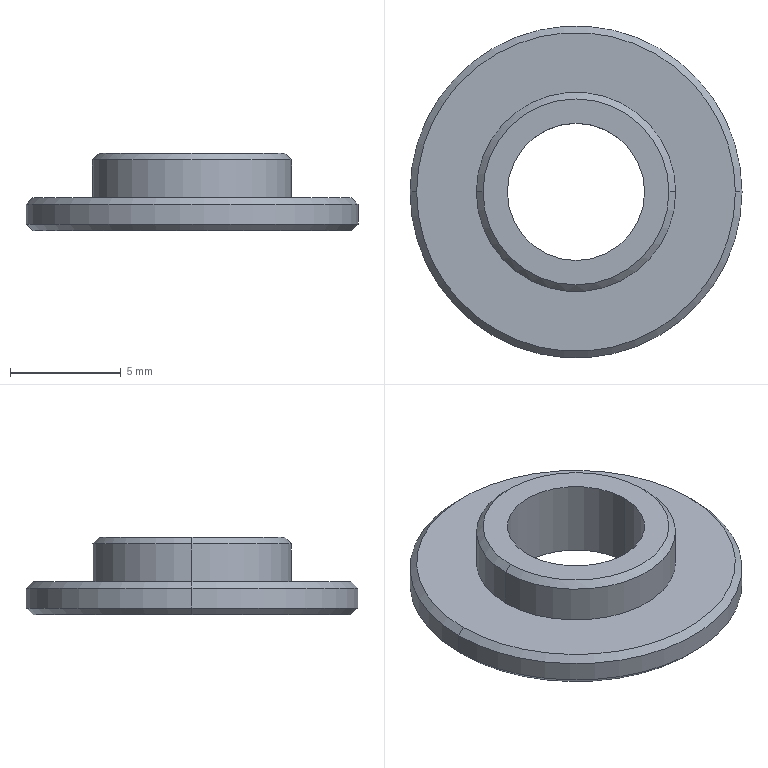Part | STEP file | 25 small sprocket spacer | 1 solid | 15 faces | box 15 x 15 x 3.5 mm | volume 281.21 mm3 | cone 6 | cylinder 6 | plane 3 | commonest cylinder face diameters 6.2 x2 9 x2 15 x2
STEP:
#1=CARTESIAN_POINT('',(0.,0.,0.));
#2=DIRECTION('',(0.,0.,1.));
#3=DIRECTION('',(1.,0.,0.));
#4=AXIS2_PLACEMENT_3D('',#1,#2,#3);
#5=CARTESIAN_POINT('',(-7.2,0.,0.));
#6=VERTEX_POINT('',#5);
#7=CARTESIAN_POINT('',(7.2,0.,0.));
#8=VERTEX_POINT('',#7);
#9=CARTESIAN_POINT('',(0.,0.,0.));
#10=DIRECTION('',(0.,0.,-1.));
#11=DIRECTION('',(1.,0.,0.));
#12=AXIS2_PLACEMENT_3D('',#9,#10,#11);
#13=CIRCLE('',#12,7.2);
#14=CARTESIAN_POINT('',(0.,0.,0.));
#15=DIRECTION('',(0.,0.,1.));
#16=DIRECTION('',(1.,0.,0.));
#17=AXIS2_PLACEMENT_3D('',#14,#15,#16);
#18=CONICAL_SURFACE('',#17,7.2,0.7854);
#19=CARTESIAN_POINT('',(6.283,0.));
#20=DIRECTION('',(-1.,0.));
#21=VECTOR('',#20,1.);
#22=LINE('',#19,#21);
#23=(GEOMETRIC_REPRESENTATION_CONTEXT(2)PARAMETRIC_REPRESENTATION_CONTEXT()REPRESENTATION_CONTEXT('',''));
#24=DEFINITIONAL_REPRESENTATION('',(#22),#23);
#25=PCURVE('',#18,#24);
#26=CARTESIAN_POINT('',(0.,0.,0.));
#27=DIRECTION('',(0.,0.,1.));
#28=DIRECTION('',(1.,0.,0.));
#29=AXIS2_PLACEMENT_3D('',#26,#27,#28);
#30=PLANE('',#29);
#31=CARTESIAN_POINT('',(7.2,0.));
#32=CARTESIAN_POINT('',(7.2,-12.471));
#33=CARTESIAN_POINT('',(-3.6,-6.235));
#34=CARTESIAN_POINT('',(-14.4,0.));
#35=CARTESIAN_POINT('',(-3.6,6.235));
#36=CARTESIAN_POINT('',(7.2,12.471));
#37=CARTESIAN_POINT('',(7.2,0.));
#38=(BOUNDED_CURVE()B_SPLINE_CURVE(2,(#31,#32,#33,#34,#35,#36,#37),.UNSPECIFIED.,.T.,.F.)B_SPLINE_CURVE_WITH_KNOTS((1,2,2,2,2,1),(-2.094,0.,2.094,4.189,6.283,8.378),.UNSPECIFIED.)CURVE()GEOMETRIC_REPRESENTATION_ITEM()RATIONAL_B_SPLINE_CURVE((1.,0.5,1.,0.5,1.,0.5,1.))REPRESENTATION_ITEM(''));
#39=(GEOMETRIC_REPRESENTATION_CONTEXT(2)PARAMETRIC_REPRESENTATION_CONTEXT()REPRESENTATION_CONTEXT('',''));
#40=DEFINITIONAL_REPRESENTATION('',(#38),#39);
#41=PCURVE('',#30,#40);
#42=SURFACE_CURVE('',#13,(#25,#41),.PCURVE_S1.);
#43=EDGE_CURVE('',#6,#8,#42,.T.);
#44=ORIENTED_EDGE('',*,*,#43,.F.);
#45=CARTESIAN_POINT('',(-7.5,0.,0.3));
#46=VERTEX_POINT('',#45);
#47=CARTESIAN_POINT('',(-7.2,0.,0.));
#48=DIRECTION('',(-0.7071,0.,0.7071));
#49=VECTOR('',#48,1.);
#50=LINE('',#47,#49);
#51=CARTESIAN_POINT('',(3.142,0.));
#52=DIRECTION('',(0.,1.));
#53=VECTOR('',#52,1.);
#54=LINE('',#51,#53);
#55=(GEOMETRIC_REPRESENTATION_CONTEXT(2)PARAMETRIC_REPRESENTATION_CONTEXT()REPRESENTATION_CONTEXT('',''));
#56=DEFINITIONAL_REPRESENTATION('',(#54),#55);
#57=PCURVE('',#18,#56);
#58=CARTESIAN_POINT('',(0.,0.,0.));
#59=DIRECTION('',(0.,0.,1.));
#60=DIRECTION('',(1.,0.,0.));
#61=AXIS2_PLACEMENT_3D('',#58,#59,#60);
#62=CONICAL_SURFACE('',#61,7.2,0.7854);
#63=CARTESIAN_POINT('',(3.142,0.));
#64=DIRECTION('',(0.,1.));
#65=VECTOR('',#64,1.);
#66=LINE('',#63,#65);
#67=(GEOMETRIC_REPRESENTATION_CONTEXT(2)PARAMETRIC_REPRESENTATION_CONTEXT()REPRESENTATION_CONTEXT('',''));
#68=DEFINITIONAL_REPRESENTATION('',(#66),#67);
#69=PCURVE('',#62,#68);
#70=SURFACE_CURVE('',#50,(#57,#69),.PCURVE_S1.);
#71=EDGE_CURVE('',#6,#46,#70,.T.);
#72=ORIENTED_EDGE('',*,*,#71,.T.);
#73=CARTESIAN_POINT('',(7.5,0.,0.3));
#74=VERTEX_POINT('',#73);
#75=CARTESIAN_POINT('',(0.,0.,0.3));
#76=DIRECTION('',(0.,0.,1.));
#77=DIRECTION('',(1.,0.,0.));
#78=AXIS2_PLACEMENT_3D('',#75,#76,#77);
#79=CIRCLE('',#78,7.5);
#80=CARTESIAN_POINT('',(0.,0.3));
#81=DIRECTION('',(1.,0.));
#82=VECTOR('',#81,1.);
#83=LINE('',#80,#82);
#84=(GEOMETRIC_REPRESENTATION_CONTEXT(2)PARAMETRIC_REPRESENTATION_CONTEXT()REPRESENTATION_CONTEXT('',''));
#85=DEFINITIONAL_REPRESENTATION('',(#83),#84);
#86=PCURVE('',#18,#85);
#87=CARTESIAN_POINT('',(0.,0.,1.5));
#88=DIRECTION('',(0.,0.,-1.));
#89=DIRECTION('',(-1.,0.,0.));
#90=AXIS2_PLACEMENT_3D('',#87,#88,#89);
#91=CYLINDRICAL_SURFACE('',#90,7.5);
#92=CARTESIAN_POINT('',(3.142,1.2));
#93=DIRECTION('',(-1.,0.));
#94=VECTOR('',#93,1.);
#95=LINE('',#92,#94);
#96=(GEOMETRIC_REPRESENTATION_CONTEXT(2)PARAMETRIC_REPRESENTATION_CONTEXT()REPRESENTATION_CONTEXT('',''));
#97=DEFINITIONAL_REPRESENTATION('',(#95),#96);
#98=PCURVE('',#91,#97);
#99=SURFACE_CURVE('',#79,(#86,#98),.PCURVE_S1.);
#100=EDGE_CURVE('',#74,#46,#99,.T.);
#101=ORIENTED_EDGE('',*,*,#100,.F.);
#102=CARTESIAN_POINT('',(7.2,0.,0.));
#103=DIRECTION('',(0.7071,0.,0.7071));
#104=VECTOR('',#103,1.);
#105=LINE('',#102,#104);
#106=CARTESIAN_POINT('',(0.,0.));
#107=DIRECTION('',(0.,1.));
#108=VECTOR('',#107,1.);
#109=LINE('',#106,#108);
#110=(GEOMETRIC_REPRESENTATION_CONTEXT(2)PARAMETRIC_REPRESENTATION_CONTEXT()REPRESENTATION_CONTEXT('',''));
#111=DEFINITIONAL_REPRESENTATION('',(#109),#110);
#112=PCURVE('',#18,#111);
#113=CARTESIAN_POINT('',(6.283,0.));
#114=DIRECTION('',(0.,1.));
#115=VECTOR('',#114,1.);
#116=LINE('',#113,#115);
#117=(GEOMETRIC_REPRESENTATION_CONTEXT(2)PARAMETRIC_REPRESENTATION_CONTEXT()REPRESENTATION_CONTEXT('',''));
#118=DEFINITIONAL_REPRESENTATION('',(#116),#117);
#119=PCURVE('',#62,#118);
#120=SURFACE_CURVE('',#105,(#112,#119),.PCURVE_S1.);
#121=EDGE_CURVE('',#8,#74,#120,.T.);
#122=ORIENTED_EDGE('',*,*,#121,.F.);
#123=EDGE_LOOP('',(#44,#72,#101,#122));
#124=FACE_BOUND('',#123,.T.);
#125=ADVANCED_FACE('',(#124),#18,.T.);
#126=CARTESIAN_POINT('',(7.2,0.,1.5));
#127=VERTEX_POINT('',#126);
#128=CARTESIAN_POINT('',(-7.2,0.,1.5));
#129=VERTEX_POINT('',#128);
#130=CARTESIAN_POINT('',(0.,0.,1.5));
#131=DIRECTION('',(0.,0.,1.));
#132=DIRECTION('',(-1.,0.,0.));
#133=AXIS2_PLACEMENT_3D('',#130,#131,#132);
#134=CIRCLE('',#133,7.2);
#135=CARTESIAN_POINT('',(0.,0.,1.2));
#136=DIRECTION('',(0.,0.,-1.));
#137=DIRECTION('',(-1.,0.,0.));
#138=AXIS2_PLACEMENT_3D('',#135,#136,#137);
#139=CONICAL_SURFACE('',#138,7.5,0.7854);
#140=CARTESIAN_POINT('',(6.283,-0.3));
#141=DIRECTION('',(-1.,0.));
#142=VECTOR('',#141,1.);
#143=LINE('',#140,#142);
#144=(GEOMETRIC_REPRESENTATION_CONTEXT(2)PARAMETRIC_REPRESENTATION_CONTEXT()REPRESENTATION_CONTEXT('',''));
#145=DEFINITIONAL_REPRESENTATION('',(#143),#144);
#146=PCURVE('',#139,#145);
#147=CARTESIAN_POINT('',(0.,0.,1.5));
#148=DIRECTION('',(0.,0.,-1.));
#149=DIRECTION('',(-1.,0.,0.));
#150=AXIS2_PLACEMENT_3D('',#147,#148,#149);
#151=PLANE('',#150);
#152=CARTESIAN_POINT('',(7.2,0.));
#153=CARTESIAN_POINT('',(7.2,-12.471));
#154=CARTESIAN_POINT('',(-3.6,-6.235));
#155=CARTESIAN_POINT('',(-14.4,0.));
#156=CARTESIAN_POINT('',(-3.6,6.235));
#157=CARTESIAN_POINT('',(7.2,12.471));
#158=CARTESIAN_POINT('',(7.2,0.));
#159=(BOUNDED_CURVE()B_SPLINE_CURVE(2,(#152,#153,#154,#155,#156,#157,#158),.UNSPECIFIED.,.T.,.F.)B_SPLINE_CURVE_WITH_KNOTS((1,2,2,2,2,1),(-2.094,0.,2.094,4.189,6.283,8.378),.UNSPECIFIED.)CURVE()GEOMETRIC_REPRESENTATION_ITEM()RATIONAL_B_SPLINE_CURVE((1.,0.5,1.,0.5,1.,0.5,1.))REPRESENTATION_ITEM(''));
#160=(GEOMETRIC_REPRESENTATION_CONTEXT(2)PARAMETRIC_REPRESENTATION_CONTEXT()REPRESENTATION_CONTEXT('',''));
#161=DEFINITIONAL_REPRESENTATION('',(#159),#160);
#162=PCURVE('',#151,#161);
#163=SURFACE_CURVE('',#134,(#146,#162),.PCURVE_S1.);
#164=EDGE_CURVE('',#127,#129,#163,.T.);
#165=ORIENTED_EDGE('',*,*,#164,.F.);
#166=CARTESIAN_POINT('',(7.5,0.,1.2));
#167=VERTEX_POINT('',#166);
#168=CARTESIAN_POINT('',(7.5,0.,1.2));
#169=DIRECTION('',(0.7071,0.,-0.7071));
#170=VECTOR('',#169,1.);
#171=LINE('',#168,#170);
#172=CARTESIAN_POINT('',(3.142,0.));
#173=DIRECTION('',(0.,1.));
#174=VECTOR('',#173,1.);
#175=LINE('',#172,#174);
#176=(GEOMETRIC_REPRESENTATION_CONTEXT(2)PARAMETRIC_REPRESENTATION_CONTEXT()REPRESENTATION_CONTEXT('',''));
#177=DEFINITIONAL_REPRESENTATION('',(#175),#176);
#178=PCURVE('',#139,#177);
#179=CARTESIAN_POINT('',(0.,0.,1.2));
#180=DIRECTION('',(0.,0.,-1.));
#181=DIRECTION('',(-1.,0.,0.));
#182=AXIS2_PLACEMENT_3D('',#179,#180,#181);
#183=CONICAL_SURFACE('',#182,7.5,0.7854);
#184=CARTESIAN_POINT('',(3.142,0.));
#185=DIRECTION('',(0.,1.));
#186=VECTOR('',#185,1.);
#187=LINE('',#184,#186);
#188=(GEOMETRIC_REPRESENTATION_CONTEXT(2)PARAMETRIC_REPRESENTATION_CONTEXT()REPRESENTATION_CONTEXT('',''));
#189=DEFINITIONAL_REPRESENTATION('',(#187),#188);
#190=PCURVE('',#183,#189);
#191=SURFACE_CURVE('',#171,(#178,#190),.PCURVE_S1.);
#192=EDGE_CURVE('',#127,#167,#191,.T.);
#193=ORIENTED_EDGE('',*,*,#192,.T.);
#194=CARTESIAN_POINT('',(-7.5,0.,1.2));
#195=VERTEX_POINT('',#194);
#196=CARTESIAN_POINT('',(0.,0.,1.2));
#197=DIRECTION('',(0.,0.,-1.));
#198=DIRECTION('',(-1.,0.,0.));
#199=AXIS2_PLACEMENT_3D('',#196,#197,#198);
#200=CIRCLE('',#199,7.5);
#201=CARTESIAN_POINT('',(0.,0.));
#202=DIRECTION('',(1.,0.));
#203=VECTOR('',#202,1.);
#204=LINE('',#201,#203);
#205=(GEOMETRIC_REPRESENTATION_CONTEXT(2)PARAMETRIC_REPRESENTATION_CONTEXT()REPRESENTATION_CONTEXT('',''));
#206=DEFINITIONAL_REPRESENTATION('',(#204),#205);
#207=PCURVE('',#139,#206);
#208=CARTESIAN_POINT('',(0.,0.3));
#209=DIRECTION('',(1.,0.));
#210=VECTOR('',#209,1.);
#211=LINE('',#208,#210);
#212=(GEOMETRIC_REPRESENTATION_CONTEXT(2)PARAMETRIC_REPRESENTATION_CONTEXT()REPRESENTATION_CONTEXT('',''));
#213=DEFINITIONAL_REPRESENTATION('',(#211),#212);
#214=PCURVE('',#91,#213);
#215=SURFACE_CURVE('',#200,(#207,#214),.PCURVE_S1.);
#216=EDGE_CURVE('',#195,#167,#215,.T.);
#217=ORIENTED_EDGE('',*,*,#216,.F.);
#218=CARTESIAN_POINT('',(-7.5,0.,1.2));
#219=DIRECTION('',(-0.7071,0.,-0.7071));
#220=VECTOR('',#219,1.);
#221=LINE('',#218,#220);
#222=CARTESIAN_POINT('',(0.,0.));
#223=DIRECTION('',(0.,1.));
#224=VECTOR('',#223,1.);
#225=LINE('',#222,#224);
#226=(GEOMETRIC_REPRESENTATION_CONTEXT(2)PARAMETRIC_REPRESENTATION_CONTEXT()REPRESENTATION_CONTEXT('',''));
#227=DEFINITIONAL_REPRESENTATION('',(#225),#226);
#228=PCURVE('',#139,#227);
#229=CARTESIAN_POINT('',(6.283,0.));
#230=DIRECTION('',(0.,1.));
#231=VECTOR('',#230,1.);
#232=LINE('',#229,#231);
#233=(GEOMETRIC_REPRESENTATION_CONTEXT(2)PARAMETRIC_REPRESENTATION_CONTEXT()REPRESENTATION_CONTEXT('',''));
#234=DEFINITIONAL_REPRESENTATION('',(#232),#233);
#235=PCURVE('',#183,#234);
#236=SURFACE_CURVE('',#221,(#228,#235),.PCURVE_S1.);
#237=EDGE_CURVE('',#129,#195,#236,.T.);
#238=ORIENTED_EDGE('',*,*,#237,.F.);
#239=EDGE_LOOP('',(#165,#193,#217,#238));
#240=FACE_BOUND('',#239,.T.);
#241=ADVANCED_FACE('',(#240),#139,.T.);
#242=CARTESIAN_POINT('',(4.2,0.,3.5));
#243=VERTEX_POINT('',#242);
#244=CARTESIAN_POINT('',(-4.2,0.,3.5));
#245=VERTEX_POINT('',#244);
#246=CARTESIAN_POINT('',(0.,0.,3.5));
#247=DIRECTION('',(0.,0.,1.));
#248=DIRECTION('',(1.,0.,0.));
#249=AXIS2_PLACEMENT_3D('',#246,#247,#248);
#250=CIRCLE('',#249,4.2);
#251=CARTESIAN_POINT('',(0.,0.,3.5));
#252=DIRECTION('',(0.,0.,-1.));
#253=DIRECTION('',(-1.,0.,0.));
#254=AXIS2_PLACEMENT_3D('',#251,#252,#253);
#255=CONICAL_SURFACE('',#254,4.2,0.7854);
#256=CARTESIAN_POINT('',(3.142,0.));
#257=DIRECTION('',(-1.,0.));
#258=VECTOR('',#257,1.);
#259=LINE('',#256,#258);
#260=(GEOMETRIC_REPRESENTATION_CONTEXT(2)PARAMETRIC_REPRESENTATION_CONTEXT()REPRESENTATION_CONTEXT('',''));
#261=DEFINITIONAL_REPRESENTATION('',(#259),#260);
#262=PCURVE('',#255,#261);
#263=CARTESIAN_POINT('',(0.,0.,3.5));
#264=DIRECTION('',(0.,0.,1.));
#265=DIRECTION('',(1.,0.,0.));
#266=AXIS2_PLACEMENT_3D('',#263,#264,#265);
#267=PLANE('',#266);
#268=CARTESIAN_POINT('',(0.,0.));
#269=DIRECTION('',(1.,0.));
#270=AXIS2_PLACEMENT_2D('',#268,#269);
#271=CIRCLE('',#270,4.2);
#272=(GEOMETRIC_REPRESENTATION_CONTEXT(2)PARAMETRIC_REPRESENTATION_CONTEXT()REPRESENTATION_CONTEXT('',''));
#273=DEFINITIONAL_REPRESENTATION('',(#271),#272);
#274=PCURVE('',#267,#273);
#275=SURFACE_CURVE('',#250,(#262,#274),.PCURVE_S1.);
#276=EDGE_CURVE('',#243,#245,#275,.T.);
#277=ORIENTED_EDGE('',*,*,#276,.F.);
#278=CARTESIAN_POINT('',(4.5,0.,3.2));
#279=VERTEX_POINT('',#278);
#280=CARTESIAN_POINT('',(4.2,0.,3.5));
#281=DIRECTION('',(0.7071,0.,-0.7071));
#282=VECTOR('',#281,1.);
#283=LINE('',#280,#282);
#284=CARTESIAN_POINT('',(3.142,0.));
#285=DIRECTION('',(0.,1.));
#286=VECTOR('',#285,1.);
#287=LINE('',#284,#286);
#288=(GEOMETRIC_REPRESENTATION_CONTEXT(2)PARAMETRIC_REPRESENTATION_CONTEXT()REPRESENTATION_CONTEXT('',''));
#289=DEFINITIONAL_REPRESENTATION('',(#287),#288);
#290=PCURVE('',#255,#289);
#291=CARTESIAN_POINT('',(0.,0.,3.5));
#292=DIRECTION('',(0.,0.,-1.));
#293=DIRECTION('',(-1.,0.,0.));
#294=AXIS2_PLACEMENT_3D('',#291,#292,#293);
#295=CONICAL_SURFACE('',#294,4.2,0.7854);
#296=CARTESIAN_POINT('',(3.142,0.));
#297=DIRECTION('',(0.,1.));
#298=VECTOR('',#297,1.);
#299=LINE('',#296,#298);
#300=(GEOMETRIC_REPRESENTATION_CONTEXT(2)PARAMETRIC_REPRESENTATION_CONTEXT()REPRESENTATION_CONTEXT('',''));
#301=DEFINITIONAL_REPRESENTATION('',(#299),#300);
#302=PCURVE('',#295,#301);
#303=SURFACE_CURVE('',#283,(#290,#302),.PCURVE_S1.);
#304=EDGE_CURVE('',#243,#279,#303,.T.);
#305=ORIENTED_EDGE('',*,*,#304,.T.);
#306=CARTESIAN_POINT('',(-4.5,0.,3.2));
#307=VERTEX_POINT('',#306);
#308=CARTESIAN_POINT('',(0.,0.,3.2));
#309=DIRECTION('',(0.,0.,-1.));
#310=DIRECTION('',(1.,0.,0.));
#311=AXIS2_PLACEMENT_3D('',#308,#309,#310);
#312=CIRCLE('',#311,4.5);
#313=CARTESIAN_POINT('',(-3.142,0.3));
#314=DIRECTION('',(1.,0.));
#315=VECTOR('',#314,1.);
#316=LINE('',#313,#315);
#317=(GEOMETRIC_REPRESENTATION_CONTEXT(2)PARAMETRIC_REPRESENTATION_CONTEXT()REPRESENTATION_CONTEXT('',''));
#318=DEFINITIONAL_REPRESENTATION('',(#316),#317);
#319=PCURVE('',#255,#318);
#320=CARTESIAN_POINT('',(0.,0.,3.5));
#321=DIRECTION('',(0.,0.,-1.));
#322=DIRECTION('',(-1.,0.,0.));
#323=AXIS2_PLACEMENT_3D('',#320,#321,#322);
#324=CYLINDRICAL_SURFACE('',#323,4.5);
#325=CARTESIAN_POINT('',(-3.142,0.3));
#326=DIRECTION('',(1.,0.));
#327=VECTOR('',#326,1.);
#328=LINE('',#325,#327);
#329=(GEOMETRIC_REPRESENTATION_CONTEXT(2)PARAMETRIC_REPRESENTATION_CONTEXT()REPRESENTATION_CONTEXT('',''));
#330=DEFINITIONAL_REPRESENTATION('',(#328),#329);
#331=PCURVE('',#324,#330);
#332=SURFACE_CURVE('',#312,(#319,#331),.PCURVE_S1.);
#333=EDGE_CURVE('',#307,#279,#332,.T.);
#334=ORIENTED_EDGE('',*,*,#333,.F.);
#335=CARTESIAN_POINT('',(-4.2,0.,3.5));
#336=DIRECTION('',(-0.7071,0.,-0.7071));
#337=VECTOR('',#336,1.);
#338=LINE('',#335,#337);
#339=CARTESIAN_POINT('',(0.,0.));
#340=DIRECTION('',(0.,1.));
#341=VECTOR('',#340,1.);
#342=LINE('',#339,#341);
#343=(GEOMETRIC_REPRESENTATION_CONTEXT(2)PARAMETRIC_REPRESENTATION_CONTEXT()REPRESENTATION_CONTEXT('',''));
#344=DEFINITIONAL_REPRESENTATION('',(#342),#343);
#345=PCURVE('',#255,#344);
#346=CARTESIAN_POINT('',(6.283,0.));
#347=DIRECTION('',(0.,1.));
#348=VECTOR('',#347,1.);
#349=LINE('',#346,#348);
#350=(GEOMETRIC_REPRESENTATION_CONTEXT(2)PARAMETRIC_REPRESENTATION_CONTEXT()REPRESENTATION_CONTEXT('',''));
#351=DEFINITIONAL_REPRESENTATION('',(#349),#350);
#352=PCURVE('',#295,#351);
#353=SURFACE_CURVE('',#338,(#345,#352),.PCURVE_S1.);
#354=EDGE_CURVE('',#245,#307,#353,.T.);
#355=ORIENTED_EDGE('',*,*,#354,.F.);
#356=EDGE_LOOP('',(#277,#305,#334,#355));
#357=FACE_BOUND('',#356,.T.);
#358=ADVANCED_FACE('',(#357),#255,.T.);
#359=ORIENTED_EDGE('',*,*,#216,.T.);
#360=CARTESIAN_POINT('',(7.5,0.,1.5));
#361=DIRECTION('',(0.,0.,-1.));
#362=VECTOR('',#361,1.);
#363=LINE('',#360,#362);
#364=CARTESIAN_POINT('',(3.142,0.));
#365=DIRECTION('',(0.,1.));
#366=VECTOR('',#365,1.);
#367=LINE('',#364,#366);
#368=(GEOMETRIC_REPRESENTATION_CONTEXT(2)PARAMETRIC_REPRESENTATION_CONTEXT()REPRESENTATION_CONTEXT('',''));
#369=DEFINITIONAL_REPRESENTATION('',(#367),#368);
#370=PCURVE('',#91,#369);
#371=CARTESIAN_POINT('',(0.,0.,1.5));
#372=DIRECTION('',(0.,0.,-1.));
#373=DIRECTION('',(-1.,0.,0.));
#374=AXIS2_PLACEMENT_3D('',#371,#372,#373);
#375=CYLINDRICAL_SURFACE('',#374,7.5);
#376=CARTESIAN_POINT('',(3.142,0.));
#377=DIRECTION('',(0.,1.));
#378=VECTOR('',#377,1.);
#379=LINE('',#376,#378);
#380=(GEOMETRIC_REPRESENTATION_CONTEXT(2)PARAMETRIC_REPRESENTATION_CONTEXT()REPRESENTATION_CONTEXT('',''));
#381=DEFINITIONAL_REPRESENTATION('',(#379),#380);
#382=PCURVE('',#375,#381);
#383=SURFACE_CURVE('',#363,(#370,#382),.PCURVE_S1.);
#384=EDGE_CURVE('',#167,#74,#383,.T.);
#385=ORIENTED_EDGE('',*,*,#384,.T.);
#386=ORIENTED_EDGE('',*,*,#100,.T.);
#387=CARTESIAN_POINT('',(-7.5,0.,1.5));
#388=DIRECTION('',(0.,0.,-1.));
#389=VECTOR('',#388,1.);
#390=LINE('',#387,#389);
#391=CARTESIAN_POINT('',(0.,0.));
#392=DIRECTION('',(0.,1.));
#393=VECTOR('',#392,1.);
#394=LINE('',#391,#393);
#395=(GEOMETRIC_REPRESENTATION_CONTEXT(2)PARAMETRIC_REPRESENTATION_CONTEXT()REPRESENTATION_CONTEXT('',''));
#396=DEFINITIONAL_REPRESENTATION('',(#394),#395);
#397=PCURVE('',#91,#396);
#398=CARTESIAN_POINT('',(6.283,0.));
#399=DIRECTION('',(0.,1.));
#400=VECTOR('',#399,1.);
#401=LINE('',#398,#400);
#402=(GEOMETRIC_REPRESENTATION_CONTEXT(2)PARAMETRIC_REPRESENTATION_CONTEXT()REPRESENTATION_CONTEXT('',''));
#403=DEFINITIONAL_REPRESENTATION('',(#401),#402);
#404=PCURVE('',#375,#403);
#405=SURFACE_CURVE('',#390,(#397,#404),.PCURVE_S1.);
#406=EDGE_CURVE('',#195,#46,#405,.T.);
#407=ORIENTED_EDGE('',*,*,#406,.F.);
#408=EDGE_LOOP('',(#359,#385,#386,#407));
#409=FACE_BOUND('',#408,.T.);
#410=ADVANCED_FACE('',(#409),#91,.T.);
#411=CARTESIAN_POINT('',(-3.1,0.,3.5));
#412=VERTEX_POINT('',#411);
#413=CARTESIAN_POINT('',(-3.1,0.,0.));
#414=VERTEX_POINT('',#413);
#415=CARTESIAN_POINT('',(-3.1,0.,3.5));
#416=DIRECTION('',(0.,0.,-1.));
#417=VECTOR('',#416,1.);
#418=LINE('',#415,#417);
#419=CARTESIAN_POINT('',(0.,0.,3.5));
#420=DIRECTION('',(0.,0.,-1.));
#421=DIRECTION('',(-1.,0.,0.));
#422=AXIS2_PLACEMENT_3D('',#419,#420,#421);
#423=CYLINDRICAL_SURFACE('',#422,3.1);
#424=CARTESIAN_POINT('',(6.283,0.));
#425=DIRECTION('',(0.,1.));
#426=VECTOR('',#425,1.);
#427=LINE('',#424,#426);
#428=(GEOMETRIC_REPRESENTATION_CONTEXT(2)PARAMETRIC_REPRESENTATION_CONTEXT()REPRESENTATION_CONTEXT('',''));
#429=DEFINITIONAL_REPRESENTATION('',(#427),#428);
#430=PCURVE('',#423,#429);
#431=CARTESIAN_POINT('',(0.,0.,3.5));
#432=DIRECTION('',(0.,0.,-1.));
#433=DIRECTION('',(-1.,0.,0.));
#434=AXIS2_PLACEMENT_3D('',#431,#432,#433);
#435=CYLINDRICAL_SURFACE('',#434,3.1);
#436=CARTESIAN_POINT('',(0.,0.));
#437=DIRECTION('',(0.,1.));
#438=VECTOR('',#437,1.);
#439=LINE('',#436,#438);
#440=(GEOMETRIC_REPRESENTATION_CONTEXT(2)PARAMETRIC_REPRESENTATION_CONTEXT()REPRESENTATION_CONTEXT('',''));
#441=DEFINITIONAL_REPRESENTATION('',(#439),#440);
#442=PCURVE('',#435,#441);
#443=SURFACE_CURVE('',#418,(#430,#442),.PCURVE_S1.);
#444=EDGE_CURVE('',#412,#414,#443,.T.);
#445=ORIENTED_EDGE('',*,*,#444,.T.);
#446=CARTESIAN_POINT('',(3.1,0.,0.));
#447=VERTEX_POINT('',#446);
#448=CARTESIAN_POINT('',(0.,0.,0.));
#449=DIRECTION('',(0.,0.,1.));
#450=DIRECTION('',(1.,0.,0.));
#451=AXIS2_PLACEMENT_3D('',#448,#449,#450);
#452=CIRCLE('',#451,3.1);
#453=CARTESIAN_POINT('',(9.425,3.5));
#454=DIRECTION('',(-1.,0.));
#455=VECTOR('',#454,1.);
#456=LINE('',#453,#455);
#457=(GEOMETRIC_REPRESENTATION_CONTEXT(2)PARAMETRIC_REPRESENTATION_CONTEXT()REPRESENTATION_CONTEXT('',''));
#458=DEFINITIONAL_REPRESENTATION('',(#456),#457);
#459=PCURVE('',#423,#458);
#460=CARTESIAN_POINT('',(0.,0.));
#461=DIRECTION('',(1.,0.));
#462=AXIS2_PLACEMENT_2D('',#460,#461);
#463=CIRCLE('',#462,3.1);
#464=(GEOMETRIC_REPRESENTATION_CONTEXT(2)PARAMETRIC_REPRESENTATION_CONTEXT()REPRESENTATION_CONTEXT('',''));
#465=DEFINITIONAL_REPRESENTATION('',(#463),#464);
#466=PCURVE('',#30,#465);
#467=SURFACE_CURVE('',#452,(#459,#466),.PCURVE_S1.);
#468=EDGE_CURVE('',#414,#447,#467,.T.);
#469=ORIENTED_EDGE('',*,*,#468,.T.);
#470=CARTESIAN_POINT('',(3.1,0.,3.5));
#471=VERTEX_POINT('',#470);
#472=CARTESIAN_POINT('',(3.1,0.,3.5));
#473=DIRECTION('',(0.,0.,-1.));
#474=VECTOR('',#473,1.);
#475=LINE('',#472,#474);
#476=CARTESIAN_POINT('',(3.142,0.));
#477=DIRECTION('',(0.,1.));
#478=VECTOR('',#477,1.);
#479=LINE('',#476,#478);
#480=(GEOMETRIC_REPRESENTATION_CONTEXT(2)PARAMETRIC_REPRESENTATION_CONTEXT()REPRESENTATION_CONTEXT('',''));
#481=DEFINITIONAL_REPRESENTATION('',(#479),#480);
#482=PCURVE('',#423,#481);
#483=CARTESIAN_POINT('',(3.142,0.));
#484=DIRECTION('',(0.,1.));
#485=VECTOR('',#484,1.);
#486=LINE('',#483,#485);
#487=(GEOMETRIC_REPRESENTATION_CONTEXT(2)PARAMETRIC_REPRESENTATION_CONTEXT()REPRESENTATION_CONTEXT('',''));
#488=DEFINITIONAL_REPRESENTATION('',(#486),#487);
#489=PCURVE('',#435,#488);
#490=SURFACE_CURVE('',#475,(#482,#489),.PCURVE_S1.);
#491=EDGE_CURVE('',#471,#447,#490,.T.);
#492=ORIENTED_EDGE('',*,*,#491,.F.);
#493=CARTESIAN_POINT('',(0.,0.,3.5));
#494=DIRECTION('',(0.,0.,1.));
#495=DIRECTION('',(1.,0.,0.));
#496=AXIS2_PLACEMENT_3D('',#493,#494,#495);
#497=CIRCLE('',#496,3.1);
#498=CARTESIAN_POINT('',(9.425,0.));
#499=DIRECTION('',(-1.,0.));
#500=VECTOR('',#499,1.);
#501=LINE('',#498,#500);
#502=(GEOMETRIC_REPRESENTATION_CONTEXT(2)PARAMETRIC_REPRESENTATION_CONTEXT()REPRESENTATION_CONTEXT('',''));
#503=DEFINITIONAL_REPRESENTATION('',(#501),#502);
#504=PCURVE('',#423,#503);
#505=CARTESIAN_POINT('',(0.,0.));
#506=DIRECTION('',(1.,0.));
#507=AXIS2_PLACEMENT_2D('',#505,#506);
#508=CIRCLE('',#507,3.1);
#509=(GEOMETRIC_REPRESENTATION_CONTEXT(2)PARAMETRIC_REPRESENTATION_CONTEXT()REPRESENTATION_CONTEXT('',''));
#510=DEFINITIONAL_REPRESENTATION('',(#508),#509);
#511=PCURVE('',#267,#510);
#512=SURFACE_CURVE('',#497,(#504,#511),.PCURVE_S1.);
#513=EDGE_CURVE('',#412,#471,#512,.T.);
#514=ORIENTED_EDGE('',*,*,#513,.F.);
#515=EDGE_LOOP('',(#445,#469,#492,#514));
#516=FACE_BOUND('',#515,.F.);
#517=ADVANCED_FACE('',(#516),#423,.F.);
#518=ORIENTED_EDGE('',*,*,#333,.T.);
#519=CARTESIAN_POINT('',(4.5,0.,1.5));
#520=VERTEX_POINT('',#519);
#521=CARTESIAN_POINT('',(4.5,0.,3.5));
#522=DIRECTION('',(0.,0.,-1.));
#523=VECTOR('',#522,1.);
#524=LINE('',#521,#523);
#525=CARTESIAN_POINT('',(3.142,0.));
#526=DIRECTION('',(0.,1.));
#527=VECTOR('',#526,1.);
#528=LINE('',#525,#527);
#529=(GEOMETRIC_REPRESENTATION_CONTEXT(2)PARAMETRIC_REPRESENTATION_CONTEXT()REPRESENTATION_CONTEXT('',''));
#530=DEFINITIONAL_REPRESENTATION('',(#528),#529);
#531=PCURVE('',#324,#530);
#532=CARTESIAN_POINT('',(0.,0.,3.5));
#533=DIRECTION('',(0.,0.,-1.));
#534=DIRECTION('',(-1.,0.,0.));
#535=AXIS2_PLACEMENT_3D('',#532,#533,#534);
#536=CYLINDRICAL_SURFACE('',#535,4.5);
#537=CARTESIAN_POINT('',(3.142,0.));
#538=DIRECTION('',(0.,1.));
#539=VECTOR('',#538,1.);
#540=LINE('',#537,#539);
#541=(GEOMETRIC_REPRESENTATION_CONTEXT(2)PARAMETRIC_REPRESENTATION_CONTEXT()REPRESENTATION_CONTEXT('',''));
#542=DEFINITIONAL_REPRESENTATION('',(#540),#541);
#543=PCURVE('',#536,#542);
#544=SURFACE_CURVE('',#524,(#531,#543),.PCURVE_S1.);
#545=EDGE_CURVE('',#279,#520,#544,.T.);
#546=ORIENTED_EDGE('',*,*,#545,.T.);
#547=CARTESIAN_POINT('',(-4.5,0.,1.5));
#548=VERTEX_POINT('',#547);
#549=CARTESIAN_POINT('',(0.,0.,1.5));
#550=DIRECTION('',(0.,0.,-1.));
#551=DIRECTION('',(-1.,0.,0.));
#552=AXIS2_PLACEMENT_3D('',#549,#550,#551);
#553=CIRCLE('',#552,4.5);
#554=CARTESIAN_POINT('',(0.,2.));
#555=DIRECTION('',(1.,0.));
#556=VECTOR('',#555,1.);
#557=LINE('',#554,#556);
#558=(GEOMETRIC_REPRESENTATION_CONTEXT(2)PARAMETRIC_REPRESENTATION_CONTEXT()REPRESENTATION_CONTEXT('',''));
#559=DEFINITIONAL_REPRESENTATION('',(#557),#558);
#560=PCURVE('',#324,#559);
#561=CARTESIAN_POINT('',(0.,0.));
#562=DIRECTION('',(1.,0.));
#563=AXIS2_PLACEMENT_2D('',#561,#562);
#564=CIRCLE('',#563,4.5);
#565=(GEOMETRIC_REPRESENTATION_CONTEXT(2)PARAMETRIC_REPRESENTATION_CONTEXT()REPRESENTATION_CONTEXT('',''));
#566=DEFINITIONAL_REPRESENTATION('',(#564),#565);
#567=PCURVE('',#151,#566);
#568=SURFACE_CURVE('',#553,(#560,#567),.PCURVE_S1.);
#569=EDGE_CURVE('',#548,#520,#568,.T.);
#570=ORIENTED_EDGE('',*,*,#569,.F.);
#571=CARTESIAN_POINT('',(-4.5,0.,3.5));
#572=DIRECTION('',(0.,0.,-1.));
#573=VECTOR('',#572,1.);
#574=LINE('',#571,#573);
#575=CARTESIAN_POINT('',(0.,0.));
#576=DIRECTION('',(0.,1.));
#577=VECTOR('',#576,1.);
#578=LINE('',#575,#577);
#579=(GEOMETRIC_REPRESENTATION_CONTEXT(2)PARAMETRIC_REPRESENTATION_CONTEXT()REPRESENTATION_CONTEXT('',''));
#580=DEFINITIONAL_REPRESENTATION('',(#578),#579);
#581=PCURVE('',#324,#580);
#582=CARTESIAN_POINT('',(6.283,0.));
#583=DIRECTION('',(0.,1.));
#584=VECTOR('',#583,1.);
#585=LINE('',#582,#584);
#586=(GEOMETRIC_REPRESENTATION_CONTEXT(2)PARAMETRIC_REPRESENTATION_CONTEXT()REPRESENTATION_CONTEXT('',''));
#587=DEFINITIONAL_REPRESENTATION('',(#585),#586);
#588=PCURVE('',#536,#587);
#589=SURFACE_CURVE('',#574,(#581,#588),.PCURVE_S1.);
#590=EDGE_CURVE('',#307,#548,#589,.T.);
#591=ORIENTED_EDGE('',*,*,#590,.F.);
#592=EDGE_LOOP('',(#518,#546,#570,#591));
#593=FACE_BOUND('',#592,.T.);
#594=ADVANCED_FACE('',(#593),#324,.T.);
#595=ORIENTED_EDGE('',*,*,#545,.F.);
#596=CARTESIAN_POINT('',(0.,0.,3.2));
#597=DIRECTION('',(0.,0.,-1.));
#598=DIRECTION('',(1.,0.,0.));
#599=AXIS2_PLACEMENT_3D('',#596,#597,#598);
#600=CIRCLE('',#599,4.5);
#601=CARTESIAN_POINT('',(3.142,0.3));
#602=DIRECTION('',(1.,0.));
#603=VECTOR('',#602,1.);
#604=LINE('',#601,#603);
#605=(GEOMETRIC_REPRESENTATION_CONTEXT(2)PARAMETRIC_REPRESENTATION_CONTEXT()REPRESENTATION_CONTEXT('',''));
#606=DEFINITIONAL_REPRESENTATION('',(#604),#605);
#607=PCURVE('',#536,#606);
#608=CARTESIAN_POINT('',(3.142,0.3));
#609=DIRECTION('',(1.,0.));
#610=VECTOR('',#609,1.);
#611=LINE('',#608,#610);
#612=(GEOMETRIC_REPRESENTATION_CONTEXT(2)PARAMETRIC_REPRESENTATION_CONTEXT()REPRESENTATION_CONTEXT('',''));
#613=DEFINITIONAL_REPRESENTATION('',(#611),#612);
#614=PCURVE('',#295,#613);
#615=SURFACE_CURVE('',#600,(#607,#614),.PCURVE_S1.);
#616=EDGE_CURVE('',#279,#307,#615,.T.);
#617=ORIENTED_EDGE('',*,*,#616,.T.);
#618=ORIENTED_EDGE('',*,*,#590,.T.);
#619=CARTESIAN_POINT('',(0.,0.,1.5));
#620=DIRECTION('',(0.,0.,-1.));
#621=DIRECTION('',(-1.,0.,0.));
#622=AXIS2_PLACEMENT_3D('',#619,#620,#621);
#623=CIRCLE('',#622,4.5);
#624=CARTESIAN_POINT('',(0.,2.));
#625=DIRECTION('',(1.,0.));
#626=VECTOR('',#625,1.);
#627=LINE('',#624,#626);
#628=(GEOMETRIC_REPRESENTATION_CONTEXT(2)PARAMETRIC_REPRESENTATION_CONTEXT()REPRESENTATION_CONTEXT('',''));
#629=DEFINITIONAL_REPRESENTATION('',(#627),#628);
#630=PCURVE('',#536,#629);
#631=CARTESIAN_POINT('',(0.,0.));
#632=DIRECTION('',(1.,0.));
#633=AXIS2_PLACEMENT_2D('',#631,#632);
#634=CIRCLE('',#633,4.5);
#635=(GEOMETRIC_REPRESENTATION_CONTEXT(2)PARAMETRIC_REPRESENTATION_CONTEXT()REPRESENTATION_CONTEXT('',''));
#636=DEFINITIONAL_REPRESENTATION('',(#634),#635);
#637=PCURVE('',#151,#636);
#638=SURFACE_CURVE('',#623,(#630,#637),.PCURVE_S1.);
#639=EDGE_CURVE('',#520,#548,#638,.T.);
#640=ORIENTED_EDGE('',*,*,#639,.F.);
#641=EDGE_LOOP('',(#595,#617,#618,#640));
#642=FACE_BOUND('',#641,.T.);
#643=ADVANCED_FACE('',(#642),#536,.T.);
#644=CARTESIAN_POINT('',(0.,0.,3.5));
#645=DIRECTION('',(0.,0.,1.));
#646=DIRECTION('',(1.,0.,0.));
#647=AXIS2_PLACEMENT_3D('',#644,#645,#646);
#648=CIRCLE('',#647,4.2);
#649=CARTESIAN_POINT('',(0.,0.));
#650=DIRECTION('',(1.,0.));
#651=AXIS2_PLACEMENT_2D('',#649,#650);
#652=CIRCLE('',#651,4.2);
#653=(GEOMETRIC_REPRESENTATION_CONTEXT(2)PARAMETRIC_REPRESENTATION_CONTEXT()REPRESENTATION_CONTEXT('',''));
#654=DEFINITIONAL_REPRESENTATION('',(#652),#653);
#655=PCURVE('',#267,#654);
#656=CARTESIAN_POINT('',(9.425,0.));
#657=DIRECTION('',(-1.,0.));
#658=VECTOR('',#657,1.);
#659=LINE('',#656,#658);
#660=(GEOMETRIC_REPRESENTATION_CONTEXT(2)PARAMETRIC_REPRESENTATION_CONTEXT()REPRESENTATION_CONTEXT('',''));
#661=DEFINITIONAL_REPRESENTATION('',(#659),#660);
#662=PCURVE('',#295,#661);
#663=SURFACE_CURVE('',#648,(#655,#662),.PCURVE_S1.);
#664=EDGE_CURVE('',#245,#243,#663,.T.);
#665=ORIENTED_EDGE('',*,*,#664,.T.);
#666=ORIENTED_EDGE('',*,*,#276,.T.);
#667=EDGE_LOOP('',(#665,#666));
#668=FACE_BOUND('',#667,.T.);
#669=ORIENTED_EDGE('',*,*,#513,.F.);
#670=CARTESIAN_POINT('',(0.,0.,3.5));
#671=DIRECTION('',(0.,0.,1.));
#672=DIRECTION('',(1.,0.,0.));
#673=AXIS2_PLACEMENT_3D('',#670,#671,#672);
#674=CIRCLE('',#673,3.1);
#675=CARTESIAN_POINT('',(0.,0.));
#676=DIRECTION('',(1.,0.));
#677=AXIS2_PLACEMENT_2D('',#675,#676);
#678=CIRCLE('',#677,3.1);
#679=(GEOMETRIC_REPRESENTATION_CONTEXT(2)PARAMETRIC_REPRESENTATION_CONTEXT()REPRESENTATION_CONTEXT('',''));
#680=DEFINITIONAL_REPRESENTATION('',(#678),#679);
#681=PCURVE('',#267,#680);
#682=CARTESIAN_POINT('',(3.142,0.));
#683=DIRECTION('',(-1.,0.));
#684=VECTOR('',#683,1.);
#685=LINE('',#682,#684);
#686=(GEOMETRIC_REPRESENTATION_CONTEXT(2)PARAMETRIC_REPRESENTATION_CONTEXT()REPRESENTATION_CONTEXT('',''));
#687=DEFINITIONAL_REPRESENTATION('',(#685),#686);
#688=PCURVE('',#435,#687);
#689=SURFACE_CURVE('',#674,(#681,#688),.PCURVE_S1.);
#690=EDGE_CURVE('',#471,#412,#689,.T.);
#691=ORIENTED_EDGE('',*,*,#690,.F.);
#692=EDGE_LOOP('',(#669,#691));
#693=FACE_BOUND('',#692,.T.);
#694=ADVANCED_FACE('',(#668,#693),#267,.T.);
#695=CARTESIAN_POINT('',(0.,0.,0.));
#696=DIRECTION('',(0.,0.,-1.));
#697=DIRECTION('',(1.,0.,0.));
#698=AXIS2_PLACEMENT_3D('',#695,#696,#697);
#699=CIRCLE('',#698,7.2);
#700=CARTESIAN_POINT('',(7.2,0.));
#701=CARTESIAN_POINT('',(7.2,-12.471));
#702=CARTESIAN_POINT('',(-3.6,-6.235));
#703=CARTESIAN_POINT('',(-14.4,0.));
#704=CARTESIAN_POINT('',(-3.6,6.235));
#705=CARTESIAN_POINT('',(7.2,12.471));
#706=CARTESIAN_POINT('',(7.2,0.));
#707=(BOUNDED_CURVE()B_SPLINE_CURVE(2,(#700,#701,#702,#703,#704,#705,#706),.UNSPECIFIED.,.T.,.F.)B_SPLINE_CURVE_WITH_KNOTS((1,2,2,2,2,1),(-2.094,0.,2.094,4.189,6.283,8.378),.UNSPECIFIED.)CURVE()GEOMETRIC_REPRESENTATION_ITEM()RATIONAL_B_SPLINE_CURVE((1.,0.5,1.,0.5,1.,0.5,1.))REPRESENTATION_ITEM(''));
#708=(GEOMETRIC_REPRESENTATION_CONTEXT(2)PARAMETRIC_REPRESENTATION_CONTEXT()REPRESENTATION_CONTEXT('',''));
#709=DEFINITIONAL_REPRESENTATION('',(#707),#708);
#710=PCURVE('',#30,#709);
#711=CARTESIAN_POINT('',(6.283,0.));
#712=DIRECTION('',(-1.,0.));
#713=VECTOR('',#712,1.);
#714=LINE('',#711,#713);
#715=(GEOMETRIC_REPRESENTATION_CONTEXT(2)PARAMETRIC_REPRESENTATION_CONTEXT()REPRESENTATION_CONTEXT('',''));
#716=DEFINITIONAL_REPRESENTATION('',(#714),#715);
#717=PCURVE('',#62,#716);
#718=SURFACE_CURVE('',#699,(#710,#717),.PCURVE_S1.);
#719=EDGE_CURVE('',#8,#6,#718,.T.);
#720=ORIENTED_EDGE('',*,*,#719,.T.);
#721=ORIENTED_EDGE('',*,*,#43,.T.);
#722=EDGE_LOOP('',(#720,#721));
#723=FACE_BOUND('',#722,.T.);
#724=ORIENTED_EDGE('',*,*,#468,.T.);
#725=CARTESIAN_POINT('',(0.,0.,0.));
#726=DIRECTION('',(0.,0.,1.));
#727=DIRECTION('',(1.,0.,0.));
#728=AXIS2_PLACEMENT_3D('',#725,#726,#727);
#729=CIRCLE('',#728,3.1);
#730=CARTESIAN_POINT('',(0.,0.));
#731=DIRECTION('',(1.,0.));
#732=AXIS2_PLACEMENT_2D('',#730,#731);
#733=CIRCLE('',#732,3.1);
#734=(GEOMETRIC_REPRESENTATION_CONTEXT(2)PARAMETRIC_REPRESENTATION_CONTEXT()REPRESENTATION_CONTEXT('',''));
#735=DEFINITIONAL_REPRESENTATION('',(#733),#734);
#736=PCURVE('',#30,#735);
#737=CARTESIAN_POINT('',(3.142,3.5));
#738=DIRECTION('',(-1.,0.));
#739=VECTOR('',#738,1.);
#740=LINE('',#737,#739);
#741=(GEOMETRIC_REPRESENTATION_CONTEXT(2)PARAMETRIC_REPRESENTATION_CONTEXT()REPRESENTATION_CONTEXT('',''));
#742=DEFINITIONAL_REPRESENTATION('',(#740),#741);
#743=PCURVE('',#435,#742);
#744=SURFACE_CURVE('',#729,(#736,#743),.PCURVE_S1.);
#745=EDGE_CURVE('',#447,#414,#744,.T.);
#746=ORIENTED_EDGE('',*,*,#745,.T.);
#747=EDGE_LOOP('',(#724,#746));
#748=FACE_BOUND('',#747,.T.);
#749=ADVANCED_FACE('',(#723,#748),#30,.F.);
#750=ORIENTED_EDGE('',*,*,#745,.T.);
#751=ORIENTED_EDGE('',*,*,#444,.F.);
#752=ORIENTED_EDGE('',*,*,#690,.F.);
#753=ORIENTED_EDGE('',*,*,#491,.T.);
#754=EDGE_LOOP('',(#750,#751,#752,#753));
#755=FACE_BOUND('',#754,.F.);
#756=ADVANCED_FACE('',(#755),#435,.F.);
#757=ORIENTED_EDGE('',*,*,#384,.F.);
#758=CARTESIAN_POINT('',(0.,0.,1.2));
#759=DIRECTION('',(0.,0.,-1.));
#760=DIRECTION('',(-1.,0.,0.));
#761=AXIS2_PLACEMENT_3D('',#758,#759,#760);
#762=CIRCLE('',#761,7.5);
#763=CARTESIAN_POINT('',(0.,0.3));
#764=DIRECTION('',(1.,0.));
#765=VECTOR('',#764,1.);
#766=LINE('',#763,#765);
#767=(GEOMETRIC_REPRESENTATION_CONTEXT(2)PARAMETRIC_REPRESENTATION_CONTEXT()REPRESENTATION_CONTEXT('',''));
#768=DEFINITIONAL_REPRESENTATION('',(#766),#767);
#769=PCURVE('',#375,#768);
#770=CARTESIAN_POINT('',(0.,0.));
#771=DIRECTION('',(1.,0.));
#772=VECTOR('',#771,1.);
#773=LINE('',#770,#772);
#774=(GEOMETRIC_REPRESENTATION_CONTEXT(2)PARAMETRIC_REPRESENTATION_CONTEXT()REPRESENTATION_CONTEXT('',''));
#775=DEFINITIONAL_REPRESENTATION('',(#773),#774);
#776=PCURVE('',#183,#775);
#777=SURFACE_CURVE('',#762,(#769,#776),.PCURVE_S1.);
#778=EDGE_CURVE('',#167,#195,#777,.T.);
#779=ORIENTED_EDGE('',*,*,#778,.T.);
#780=ORIENTED_EDGE('',*,*,#406,.T.);
#781=CARTESIAN_POINT('',(0.,0.,0.3));
#782=DIRECTION('',(0.,0.,1.));
#783=DIRECTION('',(1.,0.,0.));
#784=AXIS2_PLACEMENT_3D('',#781,#782,#783);
#785=CIRCLE('',#784,7.5);
#786=CARTESIAN_POINT('',(9.425,1.2));
#787=DIRECTION('',(-1.,0.));
#788=VECTOR('',#787,1.);
#789=LINE('',#786,#788);
#790=(GEOMETRIC_REPRESENTATION_CONTEXT(2)PARAMETRIC_REPRESENTATION_CONTEXT()REPRESENTATION_CONTEXT('',''));
#791=DEFINITIONAL_REPRESENTATION('',(#789),#790);
#792=PCURVE('',#375,#791);
#793=CARTESIAN_POINT('',(0.,0.3));
#794=DIRECTION('',(1.,0.));
#795=VECTOR('',#794,1.);
#796=LINE('',#793,#795);
#797=(GEOMETRIC_REPRESENTATION_CONTEXT(2)PARAMETRIC_REPRESENTATION_CONTEXT()REPRESENTATION_CONTEXT('',''));
#798=DEFINITIONAL_REPRESENTATION('',(#796),#797);
#799=PCURVE('',#62,#798);
#800=SURFACE_CURVE('',#785,(#792,#799),.PCURVE_S1.);
#801=EDGE_CURVE('',#46,#74,#800,.T.);
#802=ORIENTED_EDGE('',*,*,#801,.T.);
#803=EDGE_LOOP('',(#757,#779,#780,#802));
#804=FACE_BOUND('',#803,.T.);
#805=ADVANCED_FACE('',(#804),#375,.T.);
#806=CARTESIAN_POINT('',(0.,0.,1.5));
#807=DIRECTION('',(0.,0.,1.));
#808=DIRECTION('',(-1.,0.,0.));
#809=AXIS2_PLACEMENT_3D('',#806,#807,#808);
#810=CIRCLE('',#809,7.2);
#811=CARTESIAN_POINT('',(7.2,0.));
#812=CARTESIAN_POINT('',(7.2,-12.471));
#813=CARTESIAN_POINT('',(-3.6,-6.235));
#814=CARTESIAN_POINT('',(-14.4,0.));
#815=CARTESIAN_POINT('',(-3.6,6.235));
#816=CARTESIAN_POINT('',(7.2,12.471));
#817=CARTESIAN_POINT('',(7.2,0.));
#818=(BOUNDED_CURVE()B_SPLINE_CURVE(2,(#811,#812,#813,#814,#815,#816,#817),.UNSPECIFIED.,.T.,.F.)B_SPLINE_CURVE_WITH_KNOTS((1,2,2,2,2,1),(-2.094,0.,2.094,4.189,6.283,8.378),.UNSPECIFIED.)CURVE()GEOMETRIC_REPRESENTATION_ITEM()RATIONAL_B_SPLINE_CURVE((1.,0.5,1.,0.5,1.,0.5,1.))REPRESENTATION_ITEM(''));
#819=(GEOMETRIC_REPRESENTATION_CONTEXT(2)PARAMETRIC_REPRESENTATION_CONTEXT()REPRESENTATION_CONTEXT('',''));
#820=DEFINITIONAL_REPRESENTATION('',(#818),#819);
#821=PCURVE('',#151,#820);
#822=CARTESIAN_POINT('',(6.283,-0.3));
#823=DIRECTION('',(-1.,0.));
#824=VECTOR('',#823,1.);
#825=LINE('',#822,#824);
#826=(GEOMETRIC_REPRESENTATION_CONTEXT(2)PARAMETRIC_REPRESENTATION_CONTEXT()REPRESENTATION_CONTEXT('',''));
#827=DEFINITIONAL_REPRESENTATION('',(#825),#826);
#828=PCURVE('',#183,#827);
#829=SURFACE_CURVE('',#810,(#821,#828),.PCURVE_S1.);
#830=EDGE_CURVE('',#129,#127,#829,.T.);
#831=ORIENTED_EDGE('',*,*,#830,.T.);
#832=ORIENTED_EDGE('',*,*,#164,.T.);
#833=EDGE_LOOP('',(#831,#832));
#834=FACE_BOUND('',#833,.T.);
#835=ORIENTED_EDGE('',*,*,#569,.T.);
#836=ORIENTED_EDGE('',*,*,#639,.T.);
#837=EDGE_LOOP('',(#835,#836));
#838=FACE_BOUND('',#837,.T.);
#839=ADVANCED_FACE('',(#834,#838),#151,.F.);
#840=ORIENTED_EDGE('',*,*,#304,.F.);
#841=ORIENTED_EDGE('',*,*,#664,.F.);
#842=ORIENTED_EDGE('',*,*,#354,.T.);
#843=ORIENTED_EDGE('',*,*,#616,.F.);
#844=EDGE_LOOP('',(#840,#841,#842,#843));
#845=FACE_BOUND('',#844,.T.);
#846=ADVANCED_FACE('',(#845),#295,.T.);
#847=ORIENTED_EDGE('',*,*,#192,.F.);
#848=ORIENTED_EDGE('',*,*,#830,.F.);
#849=ORIENTED_EDGE('',*,*,#237,.T.);
#850=ORIENTED_EDGE('',*,*,#778,.F.);
#851=EDGE_LOOP('',(#847,#848,#849,#850));
#852=FACE_BOUND('',#851,.T.);
#853=ADVANCED_FACE('',(#852),#183,.T.);
#854=ORIENTED_EDGE('',*,*,#71,.F.);
#855=ORIENTED_EDGE('',*,*,#719,.F.);
#856=ORIENTED_EDGE('',*,*,#121,.T.);
#857=ORIENTED_EDGE('',*,*,#801,.F.);
#858=EDGE_LOOP('',(#854,#855,#856,#857));
#859=FACE_BOUND('',#858,.T.);
#860=ADVANCED_FACE('',(#859),#62,.T.);
#861=CLOSED_SHELL('',(#125,#241,#358,#410,#517,#594,#643,#694,#749,#756,#805,#839,#846,#853,#860));
#862=MANIFOLD_SOLID_BREP('',#861);
#863=(LENGTH_UNIT()NAMED_UNIT(*)SI_UNIT(.MILLI.,.METRE.));
#864=UNCERTAINTY_MEASURE_WITH_UNIT(LENGTH_MEASURE(0.0000001),#863,'','');
#865=(NAMED_UNIT(*)PLANE_ANGLE_UNIT()SI_UNIT($,.RADIAN.));
#866=(NAMED_UNIT(*)SI_UNIT($,.STERADIAN.)SOLID_ANGLE_UNIT());
#867=(GEOMETRIC_REPRESENTATION_CONTEXT(3)GLOBAL_UNCERTAINTY_ASSIGNED_CONTEXT((#864))GLOBAL_UNIT_ASSIGNED_CONTEXT((#863,#865,#866))REPRESENTATION_CONTEXT('',''));
#868=ADVANCED_BREP_SHAPE_REPRESENTATION('',(#4,#862),#867);